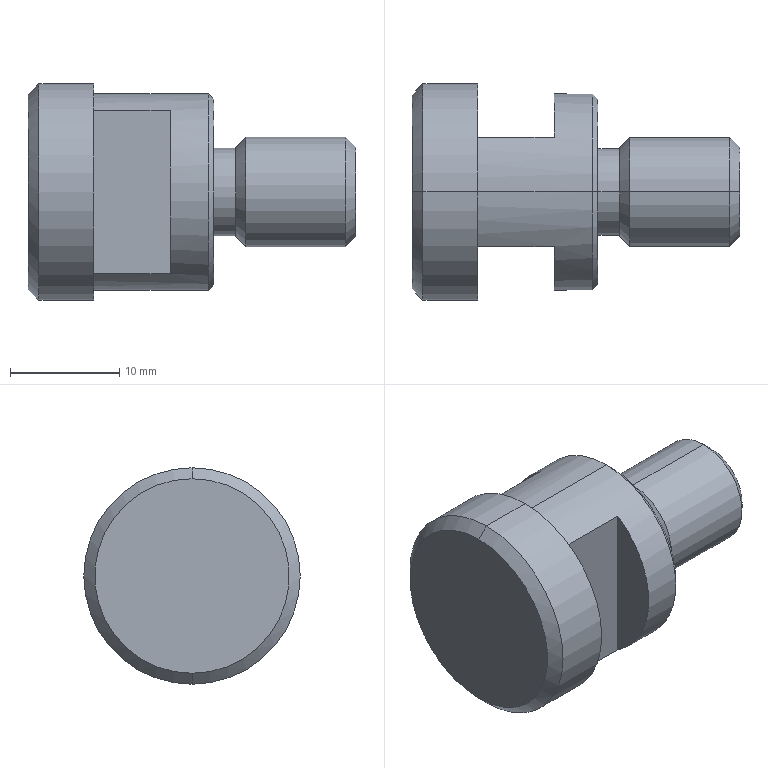Part | STEP file | _YU-05.stp | 1 solid | 25 faces | box 30 x 19.8 x 19.8 mm | volume 4960 mm3 | plane 9 | cone 8 | cylinder 8 | commonest cylinder face diameters 8 x2 10 x2 18 x2 19.8 x2